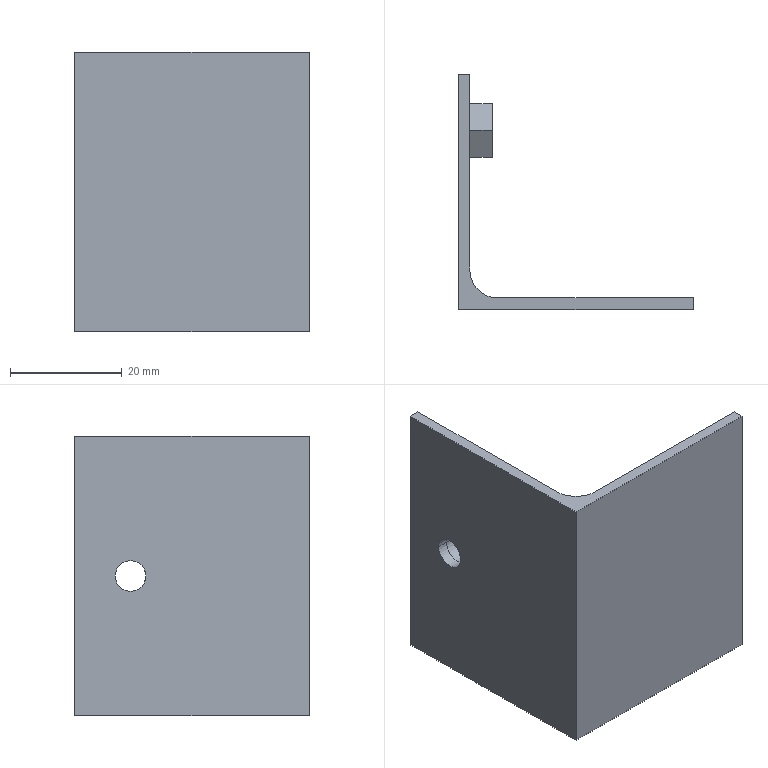Part | STEP file | ASND-0110-E63-HLTP01 control board connecting block | 2 solids | 21 faces | box 42 x 42 x 50 mm | volume 8638 mm3 | plane 16 | cylinder 5 | commonest cylinder face diameters 5.495 x2 5.5 x2 10 x1
STEP:
#1=CARTESIAN_POINT('',(0.,0.,0.));
#2=DIRECTION('',(0.,0.,1.));
#3=DIRECTION('',(1.,0.,0.));
#4=AXIS2_PLACEMENT_3D('',#1,#2,#3);
#5=CARTESIAN_POINT('',(-2.,32.75,25.));
#6=VERTEX_POINT('',#5);
#7=CARTESIAN_POINT('',(0.,32.75,25.));
#8=VERTEX_POINT('',#7);
#9=CARTESIAN_POINT('',(-10.,32.75,25.));
#10=DIRECTION('',(1.,0.,0.));
#11=VECTOR('',#10,1.);
#12=LINE('',#9,#11);
#13=CARTESIAN_POINT('',(-10.,30.,25.));
#14=DIRECTION('',(1.,0.,0.));
#15=DIRECTION('',(0.,1.,0.));
#16=AXIS2_PLACEMENT_3D('',#13,#14,#15);
#17=CYLINDRICAL_SURFACE('',#16,2.75);
#18=CARTESIAN_POINT('',(6.283,0.));
#19=DIRECTION('',(0.,1.));
#20=VECTOR('',#19,1.);
#21=LINE('',#18,#20);
#22=(GEOMETRIC_REPRESENTATION_CONTEXT(2)PARAMETRIC_REPRESENTATION_CONTEXT()REPRESENTATION_CONTEXT('',''));
#23=DEFINITIONAL_REPRESENTATION('',(#21),#22);
#24=PCURVE('',#17,#23);
#25=CARTESIAN_POINT('',(-10.,30.,25.));
#26=DIRECTION('',(1.,0.,0.));
#27=DIRECTION('',(0.,1.,0.));
#28=AXIS2_PLACEMENT_3D('',#25,#26,#27);
#29=CYLINDRICAL_SURFACE('',#28,2.75);
#30=CARTESIAN_POINT('',(0.,0.));
#31=DIRECTION('',(0.,1.));
#32=VECTOR('',#31,1.);
#33=LINE('',#30,#32);
#34=(GEOMETRIC_REPRESENTATION_CONTEXT(2)PARAMETRIC_REPRESENTATION_CONTEXT()REPRESENTATION_CONTEXT('',''));
#35=DEFINITIONAL_REPRESENTATION('',(#33),#34);
#36=PCURVE('',#29,#35);
#37=SURFACE_CURVE('',#12,(#24,#36),.PCURVE_S1.);
#38=EDGE_CURVE('',#6,#8,#37,.T.);
#39=ORIENTED_EDGE('',*,*,#38,.T.);
#40=CARTESIAN_POINT('',(0.,27.25,25.));
#41=VERTEX_POINT('',#40);
#42=CARTESIAN_POINT('',(0.,30.,25.));
#43=DIRECTION('',(1.,0.,0.));
#44=DIRECTION('',(0.,1.,0.));
#45=AXIS2_PLACEMENT_3D('',#42,#43,#44);
#46=CIRCLE('',#45,2.75);
#47=CARTESIAN_POINT('',(0.,10.));
#48=DIRECTION('',(1.,0.));
#49=VECTOR('',#48,1.);
#50=LINE('',#47,#49);
#51=(GEOMETRIC_REPRESENTATION_CONTEXT(2)PARAMETRIC_REPRESENTATION_CONTEXT()REPRESENTATION_CONTEXT('',''));
#52=DEFINITIONAL_REPRESENTATION('',(#50),#51);
#53=PCURVE('',#17,#52);
#54=CARTESIAN_POINT('',(0.,40.,50.));
#55=DIRECTION('',(1.,0.,0.));
#56=DIRECTION('',(0.,0.7071,0.7071));
#57=AXIS2_PLACEMENT_3D('',#54,#55,#56);
#58=PLANE('',#57);
#59=CARTESIAN_POINT('',(-24.749,-10.607));
#60=DIRECTION('',(0.7071,-0.7071));
#61=AXIS2_PLACEMENT_2D('',#59,#60);
#62=CIRCLE('',#61,2.75);
#63=(GEOMETRIC_REPRESENTATION_CONTEXT(2)PARAMETRIC_REPRESENTATION_CONTEXT()REPRESENTATION_CONTEXT('',''));
#64=DEFINITIONAL_REPRESENTATION('',(#62),#63);
#65=PCURVE('',#58,#64);
#66=SURFACE_CURVE('',#46,(#53,#65),.PCURVE_S1.);
#67=EDGE_CURVE('',#41,#8,#66,.T.);
#68=ORIENTED_EDGE('',*,*,#67,.F.);
#69=CARTESIAN_POINT('',(-2.,27.25,25.));
#70=VERTEX_POINT('',#69);
#71=CARTESIAN_POINT('',(-10.,27.25,25.));
#72=DIRECTION('',(1.,0.,0.));
#73=VECTOR('',#72,1.);
#74=LINE('',#71,#73);
#75=CARTESIAN_POINT('',(3.142,0.));
#76=DIRECTION('',(0.,1.));
#77=VECTOR('',#76,1.);
#78=LINE('',#75,#77);
#79=(GEOMETRIC_REPRESENTATION_CONTEXT(2)PARAMETRIC_REPRESENTATION_CONTEXT()REPRESENTATION_CONTEXT('',''));
#80=DEFINITIONAL_REPRESENTATION('',(#78),#79);
#81=PCURVE('',#17,#80);
#82=CARTESIAN_POINT('',(3.142,0.));
#83=DIRECTION('',(0.,1.));
#84=VECTOR('',#83,1.);
#85=LINE('',#82,#84);
#86=(GEOMETRIC_REPRESENTATION_CONTEXT(2)PARAMETRIC_REPRESENTATION_CONTEXT()REPRESENTATION_CONTEXT('',''));
#87=DEFINITIONAL_REPRESENTATION('',(#85),#86);
#88=PCURVE('',#29,#87);
#89=SURFACE_CURVE('',#74,(#81,#88),.PCURVE_S1.);
#90=EDGE_CURVE('',#70,#41,#89,.T.);
#91=ORIENTED_EDGE('',*,*,#90,.F.);
#92=CARTESIAN_POINT('',(-2.,30.,25.));
#93=DIRECTION('',(1.,0.,0.));
#94=DIRECTION('',(0.,1.,0.));
#95=AXIS2_PLACEMENT_3D('',#92,#93,#94);
#96=CIRCLE('',#95,2.75);
#97=CARTESIAN_POINT('',(0.,8.));
#98=DIRECTION('',(1.,0.));
#99=VECTOR('',#98,1.);
#100=LINE('',#97,#99);
#101=(GEOMETRIC_REPRESENTATION_CONTEXT(2)PARAMETRIC_REPRESENTATION_CONTEXT()REPRESENTATION_CONTEXT('',''));
#102=DEFINITIONAL_REPRESENTATION('',(#100),#101);
#103=PCURVE('',#17,#102);
#104=CARTESIAN_POINT('',(-2.,40.,50.));
#105=DIRECTION('',(1.,0.,0.));
#106=DIRECTION('',(0.,0.7071,0.7071));
#107=AXIS2_PLACEMENT_3D('',#104,#105,#106);
#108=PLANE('',#107);
#109=CARTESIAN_POINT('',(-24.749,-10.607));
#110=DIRECTION('',(0.7071,-0.7071));
#111=AXIS2_PLACEMENT_2D('',#109,#110);
#112=CIRCLE('',#111,2.75);
#113=(GEOMETRIC_REPRESENTATION_CONTEXT(2)PARAMETRIC_REPRESENTATION_CONTEXT()REPRESENTATION_CONTEXT('',''));
#114=DEFINITIONAL_REPRESENTATION('',(#112),#113);
#115=PCURVE('',#108,#114);
#116=SURFACE_CURVE('',#96,(#103,#115),.PCURVE_S1.);
#117=EDGE_CURVE('',#70,#6,#116,.T.);
#118=ORIENTED_EDGE('',*,*,#117,.T.);
#119=EDGE_LOOP('',(#39,#68,#91,#118));
#120=FACE_BOUND('',#119,.F.);
#121=ADVANCED_FACE('',(#120),#17,.F.);
#122=CARTESIAN_POINT('',(-2.,-2.,0.));
#123=VERTEX_POINT('',#122);
#124=CARTESIAN_POINT('',(40.,-2.,0.));
#125=VERTEX_POINT('',#124);
#126=CARTESIAN_POINT('',(-2.,-2.,0.));
#127=DIRECTION('',(1.,0.,0.));
#128=VECTOR('',#127,1.);
#129=LINE('',#126,#128);
#130=CARTESIAN_POINT('',(0.,-2.,50.));
#131=DIRECTION('',(0.,1.,0.));
#132=DIRECTION('',(0.7071,0.,0.7071));
#133=AXIS2_PLACEMENT_3D('',#130,#131,#132);
#134=PLANE('',#133);
#135=CARTESIAN_POINT('',(-36.77,33.941));
#136=DIRECTION('',(0.7071,0.7071));
#137=VECTOR('',#136,1.);
#138=LINE('',#135,#137);
#139=(GEOMETRIC_REPRESENTATION_CONTEXT(2)PARAMETRIC_REPRESENTATION_CONTEXT()REPRESENTATION_CONTEXT('',''));
#140=DEFINITIONAL_REPRESENTATION('',(#138),#139);
#141=PCURVE('',#134,#140);
#142=CARTESIAN_POINT('',(0.,0.,0.));
#143=DIRECTION('',(0.,0.,-1.));
#144=DIRECTION('',(0.7071,0.7071,0.));
#145=AXIS2_PLACEMENT_3D('',#142,#143,#144);
#146=PLANE('',#145);
#147=CARTESIAN_POINT('',(-2.828,0.));
#148=DIRECTION('',(0.7071,0.7071));
#149=VECTOR('',#148,1.);
#150=LINE('',#147,#149);
#151=(GEOMETRIC_REPRESENTATION_CONTEXT(2)PARAMETRIC_REPRESENTATION_CONTEXT()REPRESENTATION_CONTEXT('',''));
#152=DEFINITIONAL_REPRESENTATION('',(#150),#151);
#153=PCURVE('',#146,#152);
#154=SURFACE_CURVE('',#129,(#141,#153),.PCURVE_S1.);
#155=EDGE_CURVE('',#123,#125,#154,.T.);
#156=ORIENTED_EDGE('',*,*,#155,.T.);
#157=CARTESIAN_POINT('',(40.,-2.,50.));
#158=VERTEX_POINT('',#157);
#159=CARTESIAN_POINT('',(40.,-2.,50.));
#160=DIRECTION('',(0.,0.,-1.));
#161=VECTOR('',#160,1.);
#162=LINE('',#159,#161);
#163=CARTESIAN_POINT('',(28.284,28.284));
#164=DIRECTION('',(-0.7071,0.7071));
#165=VECTOR('',#164,1.);
#166=LINE('',#163,#165);
#167=(GEOMETRIC_REPRESENTATION_CONTEXT(2)PARAMETRIC_REPRESENTATION_CONTEXT()REPRESENTATION_CONTEXT('',''));
#168=DEFINITIONAL_REPRESENTATION('',(#166),#167);
#169=PCURVE('',#134,#168);
#170=CARTESIAN_POINT('',(40.,0.,50.));
#171=DIRECTION('',(1.,0.,0.));
#172=DIRECTION('',(0.,0.7071,0.7071));
#173=AXIS2_PLACEMENT_3D('',#170,#171,#172);
#174=PLANE('',#173);
#175=CARTESIAN_POINT('',(-1.414,1.414));
#176=DIRECTION('',(-0.7071,-0.7071));
#177=VECTOR('',#176,1.);
#178=LINE('',#175,#177);
#179=(GEOMETRIC_REPRESENTATION_CONTEXT(2)PARAMETRIC_REPRESENTATION_CONTEXT()REPRESENTATION_CONTEXT('',''));
#180=DEFINITIONAL_REPRESENTATION('',(#178),#179);
#181=PCURVE('',#174,#180);
#182=SURFACE_CURVE('',#162,(#169,#181),.PCURVE_S1.);
#183=EDGE_CURVE('',#158,#125,#182,.T.);
#184=ORIENTED_EDGE('',*,*,#183,.F.);
#185=CARTESIAN_POINT('',(-2.,-2.,50.));
#186=VERTEX_POINT('',#185);
#187=CARTESIAN_POINT('',(-2.,-2.,50.));
#188=DIRECTION('',(1.,0.,0.));
#189=VECTOR('',#188,1.);
#190=LINE('',#187,#189);
#191=CARTESIAN_POINT('',(-1.414,-1.414));
#192=DIRECTION('',(0.7071,0.7071));
#193=VECTOR('',#192,1.);
#194=LINE('',#191,#193);
#195=(GEOMETRIC_REPRESENTATION_CONTEXT(2)PARAMETRIC_REPRESENTATION_CONTEXT()REPRESENTATION_CONTEXT('',''));
#196=DEFINITIONAL_REPRESENTATION('',(#194),#195);
#197=PCURVE('',#134,#196);
#198=CARTESIAN_POINT('',(0.,0.,50.));
#199=DIRECTION('',(0.,0.,-1.));
#200=DIRECTION('',(0.7071,0.7071,0.));
#201=AXIS2_PLACEMENT_3D('',#198,#199,#200);
#202=PLANE('',#201);
#203=CARTESIAN_POINT('',(-2.828,0.));
#204=DIRECTION('',(0.7071,0.7071));
#205=VECTOR('',#204,1.);
#206=LINE('',#203,#205);
#207=(GEOMETRIC_REPRESENTATION_CONTEXT(2)PARAMETRIC_REPRESENTATION_CONTEXT()REPRESENTATION_CONTEXT('',''));
#208=DEFINITIONAL_REPRESENTATION('',(#206),#207);
#209=PCURVE('',#202,#208);
#210=SURFACE_CURVE('',#190,(#197,#209),.PCURVE_S1.);
#211=EDGE_CURVE('',#186,#158,#210,.T.);
#212=ORIENTED_EDGE('',*,*,#211,.F.);
#213=CARTESIAN_POINT('',(-2.,-2.,50.));
#214=DIRECTION('',(0.,0.,-1.));
#215=VECTOR('',#214,1.);
#216=LINE('',#213,#215);
#217=CARTESIAN_POINT('',(-1.414,-1.414));
#218=DIRECTION('',(-0.7071,0.7071));
#219=VECTOR('',#218,1.);
#220=LINE('',#217,#219);
#221=(GEOMETRIC_REPRESENTATION_CONTEXT(2)PARAMETRIC_REPRESENTATION_CONTEXT()REPRESENTATION_CONTEXT('',''));
#222=DEFINITIONAL_REPRESENTATION('',(#220),#221);
#223=PCURVE('',#134,#222);
#224=CARTESIAN_POINT('',(-29.698,29.698));
#225=DIRECTION('',(-0.7071,-0.7071));
#226=VECTOR('',#225,1.);
#227=LINE('',#224,#226);
#228=(GEOMETRIC_REPRESENTATION_CONTEXT(2)PARAMETRIC_REPRESENTATION_CONTEXT()REPRESENTATION_CONTEXT('',''));
#229=DEFINITIONAL_REPRESENTATION('',(#227),#228);
#230=PCURVE('',#108,#229);
#231=SURFACE_CURVE('',#216,(#223,#230),.PCURVE_S1.);
#232=EDGE_CURVE('',#186,#123,#231,.T.);
#233=ORIENTED_EDGE('',*,*,#232,.T.);
#234=EDGE_LOOP('',(#156,#184,#212,#233));
#235=FACE_BOUND('',#234,.T.);
#236=ADVANCED_FACE('',(#235),#134,.F.);
#237=CARTESIAN_POINT('',(40.,0.,0.));
#238=VERTEX_POINT('',#237);
#239=CARTESIAN_POINT('',(40.,0.,0.));
#240=DIRECTION('',(0.,-1.,0.));
#241=VECTOR('',#240,1.);
#242=LINE('',#239,#241);
#243=CARTESIAN_POINT('',(-35.355,-35.355));
#244=DIRECTION('',(-0.7071,0.7071));
#245=VECTOR('',#244,1.);
#246=LINE('',#243,#245);
#247=(GEOMETRIC_REPRESENTATION_CONTEXT(2)PARAMETRIC_REPRESENTATION_CONTEXT()REPRESENTATION_CONTEXT('',''));
#248=DEFINITIONAL_REPRESENTATION('',(#246),#247);
#249=PCURVE('',#174,#248);
#250=CARTESIAN_POINT('',(28.284,28.284));
#251=DIRECTION('',(-0.7071,0.7071));
#252=VECTOR('',#251,1.);
#253=LINE('',#250,#252);
#254=(GEOMETRIC_REPRESENTATION_CONTEXT(2)PARAMETRIC_REPRESENTATION_CONTEXT()REPRESENTATION_CONTEXT('',''));
#255=DEFINITIONAL_REPRESENTATION('',(#253),#254);
#256=PCURVE('',#146,#255);
#257=SURFACE_CURVE('',#242,(#249,#256),.PCURVE_S1.);
#258=EDGE_CURVE('',#238,#125,#257,.T.);
#259=ORIENTED_EDGE('',*,*,#258,.F.);
#260=CARTESIAN_POINT('',(40.,0.,50.));
#261=VERTEX_POINT('',#260);
#262=CARTESIAN_POINT('',(40.,0.,50.));
#263=DIRECTION('',(0.,0.,-1.));
#264=VECTOR('',#263,1.);
#265=LINE('',#262,#264);
#266=CARTESIAN_POINT('',(0.,0.));
#267=DIRECTION('',(-0.7071,-0.7071));
#268=VECTOR('',#267,1.);
#269=LINE('',#266,#268);
#270=(GEOMETRIC_REPRESENTATION_CONTEXT(2)PARAMETRIC_REPRESENTATION_CONTEXT()REPRESENTATION_CONTEXT('',''));
#271=DEFINITIONAL_REPRESENTATION('',(#269),#270);
#272=PCURVE('',#174,#271);
#273=CARTESIAN_POINT('',(0.,0.,50.));
#274=DIRECTION('',(0.,1.,0.));
#275=DIRECTION('',(0.7071,0.,0.7071));
#276=AXIS2_PLACEMENT_3D('',#273,#274,#275);
#277=PLANE('',#276);
#278=CARTESIAN_POINT('',(28.284,28.284));
#279=DIRECTION('',(-0.7071,0.7071));
#280=VECTOR('',#279,1.);
#281=LINE('',#278,#280);
#282=(GEOMETRIC_REPRESENTATION_CONTEXT(2)PARAMETRIC_REPRESENTATION_CONTEXT()REPRESENTATION_CONTEXT('',''));
#283=DEFINITIONAL_REPRESENTATION('',(#281),#282);
#284=PCURVE('',#277,#283);
#285=SURFACE_CURVE('',#265,(#272,#284),.PCURVE_S1.);
#286=EDGE_CURVE('',#261,#238,#285,.T.);
#287=ORIENTED_EDGE('',*,*,#286,.F.);
#288=CARTESIAN_POINT('',(40.,0.,50.));
#289=DIRECTION('',(0.,-1.,0.));
#290=VECTOR('',#289,1.);
#291=LINE('',#288,#290);
#292=CARTESIAN_POINT('',(0.,0.));
#293=DIRECTION('',(-0.7071,0.7071));
#294=VECTOR('',#293,1.);
#295=LINE('',#292,#294);
#296=(GEOMETRIC_REPRESENTATION_CONTEXT(2)PARAMETRIC_REPRESENTATION_CONTEXT()REPRESENTATION_CONTEXT('',''));
#297=DEFINITIONAL_REPRESENTATION('',(#295),#296);
#298=PCURVE('',#174,#297);
#299=CARTESIAN_POINT('',(28.284,28.284));
#300=DIRECTION('',(-0.7071,0.7071));
#301=VECTOR('',#300,1.);
#302=LINE('',#299,#301);
#303=(GEOMETRIC_REPRESENTATION_CONTEXT(2)PARAMETRIC_REPRESENTATION_CONTEXT()REPRESENTATION_CONTEXT('',''));
#304=DEFINITIONAL_REPRESENTATION('',(#302),#303);
#305=PCURVE('',#202,#304);
#306=SURFACE_CURVE('',#291,(#298,#305),.PCURVE_S1.);
#307=EDGE_CURVE('',#261,#158,#306,.T.);
#308=ORIENTED_EDGE('',*,*,#307,.T.);
#309=ORIENTED_EDGE('',*,*,#183,.T.);
#310=EDGE_LOOP('',(#259,#287,#308,#309));
#311=FACE_BOUND('',#310,.T.);
#312=ADVANCED_FACE('',(#311),#174,.T.);
#313=CARTESIAN_POINT('',(5.,0.,0.));
#314=VERTEX_POINT('',#313);
#315=CARTESIAN_POINT('',(5.,0.,0.));
#316=DIRECTION('',(1.,0.,0.));
#317=VECTOR('',#316,1.);
#318=LINE('',#315,#317);
#319=CARTESIAN_POINT('',(-31.82,38.891));
#320=DIRECTION('',(0.7071,0.7071));
#321=VECTOR('',#320,1.);
#322=LINE('',#319,#321);
#323=(GEOMETRIC_REPRESENTATION_CONTEXT(2)PARAMETRIC_REPRESENTATION_CONTEXT()REPRESENTATION_CONTEXT('',''));
#324=DEFINITIONAL_REPRESENTATION('',(#322),#323);
#325=PCURVE('',#277,#324);
#326=CARTESIAN_POINT('',(3.536,3.536));
#327=DIRECTION('',(0.7071,0.7071));
#328=VECTOR('',#327,1.);
#329=LINE('',#326,#328);
#330=(GEOMETRIC_REPRESENTATION_CONTEXT(2)PARAMETRIC_REPRESENTATION_CONTEXT()REPRESENTATION_CONTEXT('',''));
#331=DEFINITIONAL_REPRESENTATION('',(#329),#330);
#332=PCURVE('',#146,#331);
#333=SURFACE_CURVE('',#318,(#325,#332),.PCURVE_S1.);
#334=EDGE_CURVE('',#314,#238,#333,.T.);
#335=ORIENTED_EDGE('',*,*,#334,.F.);
#336=CARTESIAN_POINT('',(5.,0.,50.));
#337=VERTEX_POINT('',#336);
#338=CARTESIAN_POINT('',(5.,0.,50.));
#339=DIRECTION('',(0.,0.,1.));
#340=VECTOR('',#339,1.);
#341=LINE('',#338,#340);
#342=CARTESIAN_POINT('',(3.536,3.536));
#343=DIRECTION('',(0.7071,-0.7071));
#344=VECTOR('',#343,1.);
#345=LINE('',#342,#344);
#346=(GEOMETRIC_REPRESENTATION_CONTEXT(2)PARAMETRIC_REPRESENTATION_CONTEXT()REPRESENTATION_CONTEXT('',''));
#347=DEFINITIONAL_REPRESENTATION('',(#345),#346);
#348=PCURVE('',#277,#347);
#349=CARTESIAN_POINT('',(5.,5.,50.));
#350=DIRECTION('',(0.,0.,1.));
#351=DIRECTION('',(1.,0.,0.));
#352=AXIS2_PLACEMENT_3D('',#349,#350,#351);
#353=CYLINDRICAL_SURFACE('',#352,5.);
#354=CARTESIAN_POINT('',(4.712,0.));
#355=DIRECTION('',(0.,1.));
#356=VECTOR('',#355,1.);
#357=LINE('',#354,#356);
#358=(GEOMETRIC_REPRESENTATION_CONTEXT(2)PARAMETRIC_REPRESENTATION_CONTEXT()REPRESENTATION_CONTEXT('',''));
#359=DEFINITIONAL_REPRESENTATION('',(#357),#358);
#360=PCURVE('',#353,#359);
#361=SURFACE_CURVE('',#341,(#348,#360),.PCURVE_S1.);
#362=EDGE_CURVE('',#314,#337,#361,.T.);
#363=ORIENTED_EDGE('',*,*,#362,.T.);
#364=CARTESIAN_POINT('',(5.,0.,50.));
#365=DIRECTION('',(1.,0.,0.));
#366=VECTOR('',#365,1.);
#367=LINE('',#364,#366);
#368=CARTESIAN_POINT('',(3.536,3.536));
#369=DIRECTION('',(0.7071,0.7071));
#370=VECTOR('',#369,1.);
#371=LINE('',#368,#370);
#372=(GEOMETRIC_REPRESENTATION_CONTEXT(2)PARAMETRIC_REPRESENTATION_CONTEXT()REPRESENTATION_CONTEXT('',''));
#373=DEFINITIONAL_REPRESENTATION('',(#371),#372);
#374=PCURVE('',#277,#373);
#375=CARTESIAN_POINT('',(3.536,3.536));
#376=DIRECTION('',(0.7071,0.7071));
#377=VECTOR('',#376,1.);
#378=LINE('',#375,#377);
#379=(GEOMETRIC_REPRESENTATION_CONTEXT(2)PARAMETRIC_REPRESENTATION_CONTEXT()REPRESENTATION_CONTEXT('',''));
#380=DEFINITIONAL_REPRESENTATION('',(#378),#379);
#381=PCURVE('',#202,#380);
#382=SURFACE_CURVE('',#367,(#374,#381),.PCURVE_S1.);
#383=EDGE_CURVE('',#337,#261,#382,.T.);
#384=ORIENTED_EDGE('',*,*,#383,.T.);
#385=ORIENTED_EDGE('',*,*,#286,.T.);
#386=EDGE_LOOP('',(#335,#363,#384,#385));
#387=FACE_BOUND('',#386,.T.);
#388=ADVANCED_FACE('',(#387),#277,.T.);
#389=CARTESIAN_POINT('',(0.,40.,50.));
#390=VERTEX_POINT('',#389);
#391=CARTESIAN_POINT('',(0.,5.,50.));
#392=VERTEX_POINT('',#391);
#393=CARTESIAN_POINT('',(0.,40.,50.));
#394=DIRECTION('',(0.,-1.,0.));
#395=VECTOR('',#394,1.);
#396=LINE('',#393,#395);
#397=CARTESIAN_POINT('',(0.,0.));
#398=DIRECTION('',(-0.7071,0.7071));
#399=VECTOR('',#398,1.);
#400=LINE('',#397,#399);
#401=(GEOMETRIC_REPRESENTATION_CONTEXT(2)PARAMETRIC_REPRESENTATION_CONTEXT()REPRESENTATION_CONTEXT('',''));
#402=DEFINITIONAL_REPRESENTATION('',(#400),#401);
#403=PCURVE('',#58,#402);
#404=CARTESIAN_POINT('',(28.284,-28.284));
#405=DIRECTION('',(-0.7071,0.7071));
#406=VECTOR('',#405,1.);
#407=LINE('',#404,#406);
#408=(GEOMETRIC_REPRESENTATION_CONTEXT(2)PARAMETRIC_REPRESENTATION_CONTEXT()REPRESENTATION_CONTEXT('',''));
#409=DEFINITIONAL_REPRESENTATION('',(#407),#408);
#410=PCURVE('',#202,#409);
#411=SURFACE_CURVE('',#396,(#403,#410),.PCURVE_S1.);
#412=EDGE_CURVE('',#390,#392,#411,.T.);
#413=ORIENTED_EDGE('',*,*,#412,.T.);
#414=CARTESIAN_POINT('',(0.,5.,0.));
#415=VERTEX_POINT('',#414);
#416=CARTESIAN_POINT('',(0.,5.,50.));
#417=DIRECTION('',(0.,0.,-1.));
#418=VECTOR('',#417,1.);
#419=LINE('',#416,#418);
#420=CARTESIAN_POINT('',(-24.749,24.749));
#421=DIRECTION('',(-0.7071,-0.7071));
#422=VECTOR('',#421,1.);
#423=LINE('',#420,#422);
#424=(GEOMETRIC_REPRESENTATION_CONTEXT(2)PARAMETRIC_REPRESENTATION_CONTEXT()REPRESENTATION_CONTEXT('',''));
#425=DEFINITIONAL_REPRESENTATION('',(#423),#424);
#426=PCURVE('',#58,#425);
#427=CARTESIAN_POINT('',(3.142,0.));
#428=DIRECTION('',(0.,-1.));
#429=VECTOR('',#428,1.);
#430=LINE('',#427,#429);
#431=(GEOMETRIC_REPRESENTATION_CONTEXT(2)PARAMETRIC_REPRESENTATION_CONTEXT()REPRESENTATION_CONTEXT('',''));
#432=DEFINITIONAL_REPRESENTATION('',(#430),#431);
#433=PCURVE('',#353,#432);
#434=SURFACE_CURVE('',#419,(#426,#433),.PCURVE_S1.);
#435=EDGE_CURVE('',#392,#415,#434,.T.);
#436=ORIENTED_EDGE('',*,*,#435,.T.);
#437=CARTESIAN_POINT('',(0.,40.,0.));
#438=VERTEX_POINT('',#437);
#439=CARTESIAN_POINT('',(0.,40.,0.));
#440=DIRECTION('',(0.,-1.,0.));
#441=VECTOR('',#440,1.);
#442=LINE('',#439,#441);
#443=CARTESIAN_POINT('',(-35.355,-35.355));
#444=DIRECTION('',(-0.7071,0.7071));
#445=VECTOR('',#444,1.);
#446=LINE('',#443,#445);
#447=(GEOMETRIC_REPRESENTATION_CONTEXT(2)PARAMETRIC_REPRESENTATION_CONTEXT()REPRESENTATION_CONTEXT('',''));
#448=DEFINITIONAL_REPRESENTATION('',(#446),#447);
#449=PCURVE('',#58,#448);
#450=CARTESIAN_POINT('',(28.284,-28.284));
#451=DIRECTION('',(-0.7071,0.7071));
#452=VECTOR('',#451,1.);
#453=LINE('',#450,#452);
#454=(GEOMETRIC_REPRESENTATION_CONTEXT(2)PARAMETRIC_REPRESENTATION_CONTEXT()REPRESENTATION_CONTEXT('',''));
#455=DEFINITIONAL_REPRESENTATION('',(#453),#454);
#456=PCURVE('',#146,#455);
#457=SURFACE_CURVE('',#442,(#449,#456),.PCURVE_S1.);
#458=EDGE_CURVE('',#438,#415,#457,.T.);
#459=ORIENTED_EDGE('',*,*,#458,.F.);
#460=CARTESIAN_POINT('',(0.,40.,50.));
#461=DIRECTION('',(0.,0.,-1.));
#462=VECTOR('',#461,1.);
#463=LINE('',#460,#462);
#464=CARTESIAN_POINT('',(0.,0.));
#465=DIRECTION('',(-0.7071,-0.7071));
#466=VECTOR('',#465,1.);
#467=LINE('',#464,#466);
#468=(GEOMETRIC_REPRESENTATION_CONTEXT(2)PARAMETRIC_REPRESENTATION_CONTEXT()REPRESENTATION_CONTEXT('',''));
#469=DEFINITIONAL_REPRESENTATION('',(#467),#468);
#470=PCURVE('',#58,#469);
#471=CARTESIAN_POINT('',(-2.,40.,50.));
#472=DIRECTION('',(0.,1.,0.));
#473=DIRECTION('',(0.7071,0.,0.7071));
#474=AXIS2_PLACEMENT_3D('',#471,#472,#473);
#475=PLANE('',#474);
#476=CARTESIAN_POINT('',(1.414,1.414));
#477=DIRECTION('',(-0.7071,0.7071));
#478=VECTOR('',#477,1.);
#479=LINE('',#476,#478);
#480=(GEOMETRIC_REPRESENTATION_CONTEXT(2)PARAMETRIC_REPRESENTATION_CONTEXT()REPRESENTATION_CONTEXT('',''));
#481=DEFINITIONAL_REPRESENTATION('',(#479),#480);
#482=PCURVE('',#475,#481);
#483=SURFACE_CURVE('',#463,(#470,#482),.PCURVE_S1.);
#484=EDGE_CURVE('',#390,#438,#483,.T.);
#485=ORIENTED_EDGE('',*,*,#484,.F.);
#486=EDGE_LOOP('',(#413,#436,#459,#485));
#487=FACE_BOUND('',#486,.T.);
#488=CARTESIAN_POINT('',(0.,30.,25.));
#489=DIRECTION('',(1.,0.,0.));
#490=DIRECTION('',(0.,1.,0.));
#491=AXIS2_PLACEMENT_3D('',#488,#489,#490);
#492=CIRCLE('',#491,2.75);
#493=CARTESIAN_POINT('',(-24.749,-10.607));
#494=DIRECTION('',(0.7071,-0.7071));
#495=AXIS2_PLACEMENT_2D('',#493,#494);
#496=CIRCLE('',#495,2.75);
#497=(GEOMETRIC_REPRESENTATION_CONTEXT(2)PARAMETRIC_REPRESENTATION_CONTEXT()REPRESENTATION_CONTEXT('',''));
#498=DEFINITIONAL_REPRESENTATION('',(#496),#497);
#499=PCURVE('',#58,#498);
#500=CARTESIAN_POINT('',(0.,10.));
#501=DIRECTION('',(1.,0.));
#502=VECTOR('',#501,1.);
#503=LINE('',#500,#502);
#504=(GEOMETRIC_REPRESENTATION_CONTEXT(2)PARAMETRIC_REPRESENTATION_CONTEXT()REPRESENTATION_CONTEXT('',''));
#505=DEFINITIONAL_REPRESENTATION('',(#503),#504);
#506=PCURVE('',#29,#505);
#507=SURFACE_CURVE('',#492,(#499,#506),.PCURVE_S1.);
#508=EDGE_CURVE('',#8,#41,#507,.T.);
#509=ORIENTED_EDGE('',*,*,#508,.F.);
#510=ORIENTED_EDGE('',*,*,#67,.F.);
#511=EDGE_LOOP('',(#509,#510));
#512=FACE_BOUND('',#511,.T.);
#513=ADVANCED_FACE('',(#487,#512),#58,.T.);
#514=CARTESIAN_POINT('',(-2.,40.,0.));
#515=VERTEX_POINT('',#514);
#516=CARTESIAN_POINT('',(-2.,40.,0.));
#517=DIRECTION('',(1.,0.,0.));
#518=VECTOR('',#517,1.);
#519=LINE('',#516,#518);
#520=CARTESIAN_POINT('',(-35.355,35.355));
#521=DIRECTION('',(0.7071,0.7071));
#522=VECTOR('',#521,1.);
#523=LINE('',#520,#522);
#524=(GEOMETRIC_REPRESENTATION_CONTEXT(2)PARAMETRIC_REPRESENTATION_CONTEXT()REPRESENTATION_CONTEXT('',''));
#525=DEFINITIONAL_REPRESENTATION('',(#523),#524);
#526=PCURVE('',#475,#525);
#527=CARTESIAN_POINT('',(26.87,-29.698));
#528=DIRECTION('',(0.7071,0.7071));
#529=VECTOR('',#528,1.);
#530=LINE('',#527,#529);
#531=(GEOMETRIC_REPRESENTATION_CONTEXT(2)PARAMETRIC_REPRESENTATION_CONTEXT()REPRESENTATION_CONTEXT('',''));
#532=DEFINITIONAL_REPRESENTATION('',(#530),#531);
#533=PCURVE('',#146,#532);
#534=SURFACE_CURVE('',#519,(#526,#533),.PCURVE_S1.);
#535=EDGE_CURVE('',#515,#438,#534,.T.);
#536=ORIENTED_EDGE('',*,*,#535,.F.);
#537=CARTESIAN_POINT('',(-2.,40.,50.));
#538=VERTEX_POINT('',#537);
#539=CARTESIAN_POINT('',(-2.,40.,50.));
#540=DIRECTION('',(0.,0.,-1.));
#541=VECTOR('',#540,1.);
#542=LINE('',#539,#541);
#543=CARTESIAN_POINT('',(0.,0.));
#544=DIRECTION('',(-0.7071,0.7071));
#545=VECTOR('',#544,1.);
#546=LINE('',#543,#545);
#547=(GEOMETRIC_REPRESENTATION_CONTEXT(2)PARAMETRIC_REPRESENTATION_CONTEXT()REPRESENTATION_CONTEXT('',''));
#548=DEFINITIONAL_REPRESENTATION('',(#546),#547);
#549=PCURVE('',#475,#548);
#550=CARTESIAN_POINT('',(0.,0.));
#551=DIRECTION('',(-0.7071,-0.7071));
#552=VECTOR('',#551,1.);
#553=LINE('',#550,#552);
#554=(GEOMETRIC_REPRESENTATION_CONTEXT(2)PARAMETRIC_REPRESENTATION_CONTEXT()REPRESENTATION_CONTEXT('',''));
#555=DEFINITIONAL_REPRESENTATION('',(#553),#554);
#556=PCURVE('',#108,#555);
#557=SURFACE_CURVE('',#542,(#549,#556),.PCURVE_S1.);
#558=EDGE_CURVE('',#538,#515,#557,.T.);
#559=ORIENTED_EDGE('',*,*,#558,.F.);
#560=CARTESIAN_POINT('',(-2.,40.,50.));
#561=DIRECTION('',(1.,0.,0.));
#562=VECTOR('',#561,1.);
#563=LINE('',#560,#562);
#564=CARTESIAN_POINT('',(0.,0.));
#565=DIRECTION('',(0.7071,0.7071));
#566=VECTOR('',#565,1.);
#567=LINE('',#564,#566);
#568=(GEOMETRIC_REPRESENTATION_CONTEXT(2)PARAMETRIC_REPRESENTATION_CONTEXT()REPRESENTATION_CONTEXT('',''));
#569=DEFINITIONAL_REPRESENTATION('',(#567),#568);
#570=PCURVE('',#475,#569);
#571=CARTESIAN_POINT('',(26.87,-29.698));
#572=DIRECTION('',(0.7071,0.7071));
#573=VECTOR('',#572,1.);
#574=LINE('',#571,#573);
#575=(GEOMETRIC_REPRESENTATION_CONTEXT(2)PARAMETRIC_REPRESENTATION_CONTEXT()REPRESENTATION_CONTEXT('',''));
#576=DEFINITIONAL_REPRESENTATION('',(#574),#575);
#577=PCURVE('',#202,#576);
#578=SURFACE_CURVE('',#563,(#570,#577),.PCURVE_S1.);
#579=EDGE_CURVE('',#538,#390,#578,.T.);
#580=ORIENTED_EDGE('',*,*,#579,.T.);
#581=ORIENTED_EDGE('',*,*,#484,.T.);
#582=EDGE_LOOP('',(#536,#559,#580,#581));
#583=FACE_BOUND('',#582,.T.);
#584=ADVANCED_FACE('',(#583),#475,.T.);
#585=CARTESIAN_POINT('',(-2.,40.,0.));
#586=DIRECTION('',(0.,-1.,0.));
#587=VECTOR('',#586,1.);
#588=LINE('',#585,#587);
#589=CARTESIAN_POINT('',(-35.355,-35.355));
#590=DIRECTION('',(-0.7071,0.7071));
#591=VECTOR('',#590,1.);
#592=LINE('',#589,#591);
#593=(GEOMETRIC_REPRESENTATION_CONTEXT(2)PARAMETRIC_REPRESENTATION_CONTEXT()REPRESENTATION_CONTEXT('',''));
#594=DEFINITIONAL_REPRESENTATION('',(#592),#593);
#595=PCURVE('',#108,#594);
#596=CARTESIAN_POINT('',(26.87,-29.698));
#597=DIRECTION('',(-0.7071,0.7071));
#598=VECTOR('',#597,1.);
#599=LINE('',#596,#598);
#600=(GEOMETRIC_REPRESENTATION_CONTEXT(2)PARAMETRIC_REPRESENTATION_CONTEXT()REPRESENTATION_CONTEXT('',''));
#601=DEFINITIONAL_REPRESENTATION('',(#599),#600);
#602=PCURVE('',#146,#601);
#603=SURFACE_CURVE('',#588,(#595,#602),.PCURVE_S1.);
#604=EDGE_CURVE('',#515,#123,#603,.T.);
#605=ORIENTED_EDGE('',*,*,#604,.T.);
#606=ORIENTED_EDGE('',*,*,#232,.F.);
#607=CARTESIAN_POINT('',(-2.,40.,50.));
#608=DIRECTION('',(0.,-1.,0.));
#609=VECTOR('',#608,1.);
#610=LINE('',#607,#609);
#611=CARTESIAN_POINT('',(0.,0.));
#612=DIRECTION('',(-0.7071,0.7071));
#613=VECTOR('',#612,1.);
#614=LINE('',#611,#613);
#615=(GEOMETRIC_REPRESENTATION_CONTEXT(2)PARAMETRIC_REPRESENTATION_CONTEXT()REPRESENTATION_CONTEXT('',''));
#616=DEFINITIONAL_REPRESENTATION('',(#614),#615);
#617=PCURVE('',#108,#616);
#618=CARTESIAN_POINT('',(26.87,-29.698));
#619=DIRECTION('',(-0.7071,0.7071));
#620=VECTOR('',#619,1.);
#621=LINE('',#618,#620);
#622=(GEOMETRIC_REPRESENTATION_CONTEXT(2)PARAMETRIC_REPRESENTATION_CONTEXT()REPRESENTATION_CONTEXT('',''));
#623=DEFINITIONAL_REPRESENTATION('',(#621),#622);
#624=PCURVE('',#202,#623);
#625=SURFACE_CURVE('',#610,(#617,#624),.PCURVE_S1.);
#626=EDGE_CURVE('',#538,#186,#625,.T.);
#627=ORIENTED_EDGE('',*,*,#626,.F.);
#628=ORIENTED_EDGE('',*,*,#558,.T.);
#629=EDGE_LOOP('',(#605,#606,#627,#628));
#630=FACE_BOUND('',#629,.T.);
#631=CARTESIAN_POINT('',(-2.,30.,25.));
#632=DIRECTION('',(1.,0.,0.));
#633=DIRECTION('',(0.,1.,0.));
#634=AXIS2_PLACEMENT_3D('',#631,#632,#633);
#635=CIRCLE('',#634,2.75);
#636=CARTESIAN_POINT('',(-24.749,-10.607));
#637=DIRECTION('',(0.7071,-0.7071));
#638=AXIS2_PLACEMENT_2D('',#636,#637);
#639=CIRCLE('',#638,2.75);
#640=(GEOMETRIC_REPRESENTATION_CONTEXT(2)PARAMETRIC_REPRESENTATION_CONTEXT()REPRESENTATION_CONTEXT('',''));
#641=DEFINITIONAL_REPRESENTATION('',(#639),#640);
#642=PCURVE('',#108,#641);
#643=CARTESIAN_POINT('',(0.,8.));
#644=DIRECTION('',(1.,0.));
#645=VECTOR('',#644,1.);
#646=LINE('',#643,#645);
#647=(GEOMETRIC_REPRESENTATION_CONTEXT(2)PARAMETRIC_REPRESENTATION_CONTEXT()REPRESENTATION_CONTEXT('',''));
#648=DEFINITIONAL_REPRESENTATION('',(#646),#647);
#649=PCURVE('',#29,#648);
#650=SURFACE_CURVE('',#635,(#642,#649),.PCURVE_S1.);
#651=EDGE_CURVE('',#6,#70,#650,.T.);
#652=ORIENTED_EDGE('',*,*,#651,.T.);
#653=ORIENTED_EDGE('',*,*,#117,.T.);
#654=EDGE_LOOP('',(#652,#653));
#655=FACE_BOUND('',#654,.T.);
#656=ADVANCED_FACE('',(#630,#655),#108,.F.);
#657=ORIENTED_EDGE('',*,*,#211,.T.);
#658=ORIENTED_EDGE('',*,*,#307,.F.);
#659=ORIENTED_EDGE('',*,*,#383,.F.);
#660=CARTESIAN_POINT('',(5.,5.,50.));
#661=DIRECTION('',(0.,0.,-1.));
#662=DIRECTION('',(-1.,0.,0.));
#663=AXIS2_PLACEMENT_3D('',#660,#661,#662);
#664=CIRCLE('',#663,5.);
#665=CARTESIAN_POINT('',(7.071,0.));
#666=DIRECTION('',(-0.7071,-0.7071));
#667=AXIS2_PLACEMENT_2D('',#665,#666);
#668=CIRCLE('',#667,5.);
#669=(GEOMETRIC_REPRESENTATION_CONTEXT(2)PARAMETRIC_REPRESENTATION_CONTEXT()REPRESENTATION_CONTEXT('',''));
#670=DEFINITIONAL_REPRESENTATION('',(#668),#669);
#671=PCURVE('',#202,#670);
#672=CARTESIAN_POINT('',(9.425,0.));
#673=DIRECTION('',(-1.,0.));
#674=VECTOR('',#673,1.);
#675=LINE('',#672,#674);
#676=(GEOMETRIC_REPRESENTATION_CONTEXT(2)PARAMETRIC_REPRESENTATION_CONTEXT()REPRESENTATION_CONTEXT('',''));
#677=DEFINITIONAL_REPRESENTATION('',(#675),#676);
#678=PCURVE('',#353,#677);
#679=SURFACE_CURVE('',#664,(#671,#678),.PCURVE_S1.);
#680=EDGE_CURVE('',#337,#392,#679,.T.);
#681=ORIENTED_EDGE('',*,*,#680,.T.);
#682=ORIENTED_EDGE('',*,*,#412,.F.);
#683=ORIENTED_EDGE('',*,*,#579,.F.);
#684=ORIENTED_EDGE('',*,*,#626,.T.);
#685=EDGE_LOOP('',(#657,#658,#659,#681,#682,#683,#684));
#686=FACE_BOUND('',#685,.T.);
#687=ADVANCED_FACE('',(#686),#202,.F.);
#688=ORIENTED_EDGE('',*,*,#155,.F.);
#689=ORIENTED_EDGE('',*,*,#604,.F.);
#690=ORIENTED_EDGE('',*,*,#535,.T.);
#691=ORIENTED_EDGE('',*,*,#458,.T.);
#692=CARTESIAN_POINT('',(5.,5.,0.));
#693=DIRECTION('',(0.,0.,1.));
#694=DIRECTION('',(-1.,0.,0.));
#695=AXIS2_PLACEMENT_3D('',#692,#693,#694);
#696=CIRCLE('',#695,5.);
#697=CARTESIAN_POINT('',(3.536,-3.536));
#698=CARTESIAN_POINT('',(-2.588,2.588));
#699=CARTESIAN_POINT('',(5.777,4.83));
#700=CARTESIAN_POINT('',(14.142,7.071));
#701=CARTESIAN_POINT('',(11.901,-1.294));
#702=CARTESIAN_POINT('',(9.659,-9.659));
#703=CARTESIAN_POINT('',(3.536,-3.536));
#704=(BOUNDED_CURVE()B_SPLINE_CURVE(2,(#697,#698,#699,#700,#701,#702,#703),.UNSPECIFIED.,.T.,.F.)B_SPLINE_CURVE_WITH_KNOTS((1,2,2,2,2,1),(-2.094,0.,2.094,4.189,6.283,8.378),.UNSPECIFIED.)CURVE()GEOMETRIC_REPRESENTATION_ITEM()RATIONAL_B_SPLINE_CURVE((1.,0.5,1.,0.5,1.,0.5,1.))REPRESENTATION_ITEM(''));
#705=(GEOMETRIC_REPRESENTATION_CONTEXT(2)PARAMETRIC_REPRESENTATION_CONTEXT()REPRESENTATION_CONTEXT('',''));
#706=DEFINITIONAL_REPRESENTATION('',(#704),#705);
#707=PCURVE('',#146,#706);
#708=CARTESIAN_POINT('',(3.142,-50.));
#709=DIRECTION('',(1.,0.));
#710=VECTOR('',#709,1.);
#711=LINE('',#708,#710);
#712=(GEOMETRIC_REPRESENTATION_CONTEXT(2)PARAMETRIC_REPRESENTATION_CONTEXT()REPRESENTATION_CONTEXT('',''));
#713=DEFINITIONAL_REPRESENTATION('',(#711),#712);
#714=PCURVE('',#353,#713);
#715=SURFACE_CURVE('',#696,(#707,#714),.PCURVE_S1.);
#716=EDGE_CURVE('',#415,#314,#715,.T.);
#717=ORIENTED_EDGE('',*,*,#716,.T.);
#718=ORIENTED_EDGE('',*,*,#334,.T.);
#719=ORIENTED_EDGE('',*,*,#258,.T.);
#720=EDGE_LOOP('',(#688,#689,#690,#691,#717,#718,#719));
#721=FACE_BOUND('',#720,.T.);
#722=ADVANCED_FACE('',(#721),#146,.T.);
#723=ORIENTED_EDGE('',*,*,#435,.T.);
#724=ORIENTED_EDGE('',*,*,#716,.T.);
#725=ORIENTED_EDGE('',*,*,#362,.T.);
#726=ORIENTED_EDGE('',*,*,#680,.T.);
#727=EDGE_LOOP('',(#723,#724,#725,#726));
#728=FACE_BOUND('',#727,.F.);
#729=ADVANCED_FACE('',(#728),#353,.F.);
#730=ORIENTED_EDGE('',*,*,#508,.F.);
#731=ORIENTED_EDGE('',*,*,#38,.F.);
#732=ORIENTED_EDGE('',*,*,#651,.T.);
#733=ORIENTED_EDGE('',*,*,#90,.T.);
#734=EDGE_LOOP('',(#730,#731,#732,#733));
#735=FACE_BOUND('',#734,.F.);
#736=ADVANCED_FACE('',(#735),#29,.F.);
#737=CLOSED_SHELL('',(#121,#236,#312,#388,#513,#584,#656,#687,#722,#729,#736));
#738=MANIFOLD_SOLID_BREP('',#737);
#739=CARTESIAN_POINT('',(4.,27.253,25.));
#740=VERTEX_POINT('',#739);
#741=CARTESIAN_POINT('',(0.,27.253,25.));
#742=VERTEX_POINT('',#741);
#743=CARTESIAN_POINT('',(4.,27.253,25.));
#744=DIRECTION('',(-1.,0.,0.));
#745=VECTOR('',#744,1.);
#746=LINE('',#743,#745);
#747=CARTESIAN_POINT('',(4.,30.,25.));
#748=DIRECTION('',(-1.,0.,0.));
#749=DIRECTION('',(0.,-1.,0.));
#750=AXIS2_PLACEMENT_3D('',#747,#748,#749);
#751=CYLINDRICAL_SURFACE('',#750,2.748);
#752=CARTESIAN_POINT('',(6.283,0.));
#753=DIRECTION('',(0.,1.));
#754=VECTOR('',#753,1.);
#755=LINE('',#752,#754);
#756=(GEOMETRIC_REPRESENTATION_CONTEXT(2)PARAMETRIC_REPRESENTATION_CONTEXT()REPRESENTATION_CONTEXT('',''));
#757=DEFINITIONAL_REPRESENTATION('',(#755),#756);
#758=PCURVE('',#751,#757);
#759=CARTESIAN_POINT('',(4.,30.,25.));
#760=DIRECTION('',(-1.,0.,0.));
#761=DIRECTION('',(0.,-1.,0.));
#762=AXIS2_PLACEMENT_3D('',#759,#760,#761);
#763=CYLINDRICAL_SURFACE('',#762,2.748);
#764=CARTESIAN_POINT('',(0.,0.));
#765=DIRECTION('',(0.,1.));
#766=VECTOR('',#765,1.);
#767=LINE('',#764,#766);
#768=(GEOMETRIC_REPRESENTATION_CONTEXT(2)PARAMETRIC_REPRESENTATION_CONTEXT()REPRESENTATION_CONTEXT('',''));
#769=DEFINITIONAL_REPRESENTATION('',(#767),#768);
#770=PCURVE('',#763,#769);
#771=SURFACE_CURVE('',#746,(#758,#770),.PCURVE_S1.);
#772=EDGE_CURVE('',#740,#742,#771,.T.);
#773=ORIENTED_EDGE('',*,*,#772,.T.);
#774=CARTESIAN_POINT('',(0.,32.748,25.));
#775=VERTEX_POINT('',#774);
#776=CARTESIAN_POINT('',(0.,30.,25.));
#777=DIRECTION('',(1.,0.,0.));
#778=DIRECTION('',(0.,1.,0.));
#779=AXIS2_PLACEMENT_3D('',#776,#777,#778);
#780=CIRCLE('',#779,2.748);
#781=CARTESIAN_POINT('',(9.425,4.));
#782=DIRECTION('',(-1.,0.));
#783=VECTOR('',#782,1.);
#784=LINE('',#781,#783);
#785=(GEOMETRIC_REPRESENTATION_CONTEXT(2)PARAMETRIC_REPRESENTATION_CONTEXT()REPRESENTATION_CONTEXT('',''));
#786=DEFINITIONAL_REPRESENTATION('',(#784),#785);
#787=PCURVE('',#751,#786);
#788=CARTESIAN_POINT('',(0.,0.,0.));
#789=DIRECTION('',(1.,0.,0.));
#790=DIRECTION('',(0.,0.7071,0.7071));
#791=AXIS2_PLACEMENT_3D('',#788,#789,#790);
#792=PLANE('',#791);
#793=CARTESIAN_POINT('',(38.891,-3.536));
#794=DIRECTION('',(0.7071,-0.7071));
#795=AXIS2_PLACEMENT_2D('',#793,#794);
#796=CIRCLE('',#795,2.748);
#797=(GEOMETRIC_REPRESENTATION_CONTEXT(2)PARAMETRIC_REPRESENTATION_CONTEXT()REPRESENTATION_CONTEXT('',''));
#798=DEFINITIONAL_REPRESENTATION('',(#796),#797);
#799=PCURVE('',#792,#798);
#800=SURFACE_CURVE('',#780,(#787,#799),.PCURVE_S1.);
#801=EDGE_CURVE('',#742,#775,#800,.T.);
#802=ORIENTED_EDGE('',*,*,#801,.T.);
#803=CARTESIAN_POINT('',(4.,32.748,25.));
#804=VERTEX_POINT('',#803);
#805=CARTESIAN_POINT('',(4.,32.748,25.));
#806=DIRECTION('',(-1.,0.,0.));
#807=VECTOR('',#806,1.);
#808=LINE('',#805,#807);
#809=CARTESIAN_POINT('',(3.142,0.));
#810=DIRECTION('',(0.,1.));
#811=VECTOR('',#810,1.);
#812=LINE('',#809,#811);
#813=(GEOMETRIC_REPRESENTATION_CONTEXT(2)PARAMETRIC_REPRESENTATION_CONTEXT()REPRESENTATION_CONTEXT('',''));
#814=DEFINITIONAL_REPRESENTATION('',(#812),#813);
#815=PCURVE('',#751,#814);
#816=CARTESIAN_POINT('',(3.142,0.));
#817=DIRECTION('',(0.,1.));
#818=VECTOR('',#817,1.);
#819=LINE('',#816,#818);
#820=(GEOMETRIC_REPRESENTATION_CONTEXT(2)PARAMETRIC_REPRESENTATION_CONTEXT()REPRESENTATION_CONTEXT('',''));
#821=DEFINITIONAL_REPRESENTATION('',(#819),#820);
#822=PCURVE('',#763,#821);
#823=SURFACE_CURVE('',#808,(#815,#822),.PCURVE_S1.);
#824=EDGE_CURVE('',#804,#775,#823,.T.);
#825=ORIENTED_EDGE('',*,*,#824,.F.);
#826=CARTESIAN_POINT('',(4.,30.,25.));
#827=DIRECTION('',(1.,0.,0.));
#828=DIRECTION('',(0.,1.,0.));
#829=AXIS2_PLACEMENT_3D('',#826,#827,#828);
#830=CIRCLE('',#829,2.748);
#831=CARTESIAN_POINT('',(9.425,0.));
#832=DIRECTION('',(-1.,0.));
#833=VECTOR('',#832,1.);
#834=LINE('',#831,#833);
#835=(GEOMETRIC_REPRESENTATION_CONTEXT(2)PARAMETRIC_REPRESENTATION_CONTEXT()REPRESENTATION_CONTEXT('',''));
#836=DEFINITIONAL_REPRESENTATION('',(#834),#835);
#837=PCURVE('',#751,#836);
#838=CARTESIAN_POINT('',(4.,0.,0.));
#839=DIRECTION('',(1.,0.,0.));
#840=DIRECTION('',(0.,0.7071,0.7071));
#841=AXIS2_PLACEMENT_3D('',#838,#839,#840);
#842=PLANE('',#841);
#843=CARTESIAN_POINT('',(38.891,-3.536));
#844=DIRECTION('',(0.7071,-0.7071));
#845=AXIS2_PLACEMENT_2D('',#843,#844);
#846=CIRCLE('',#845,2.748);
#847=(GEOMETRIC_REPRESENTATION_CONTEXT(2)PARAMETRIC_REPRESENTATION_CONTEXT()REPRESENTATION_CONTEXT('',''));
#848=DEFINITIONAL_REPRESENTATION('',(#846),#847);
#849=PCURVE('',#842,#848);
#850=SURFACE_CURVE('',#830,(#837,#849),.PCURVE_S1.);
#851=EDGE_CURVE('',#740,#804,#850,.T.);
#852=ORIENTED_EDGE('',*,*,#851,.F.);
#853=EDGE_LOOP('',(#773,#802,#825,#852));
#854=FACE_BOUND('',#853,.F.);
#855=ADVANCED_FACE('',(#854),#751,.F.);
#856=CARTESIAN_POINT('',(4.,30.,19.518));
#857=VERTEX_POINT('',#856);
#858=CARTESIAN_POINT('',(4.,34.748,22.259));
#859=VERTEX_POINT('',#858);
#860=CARTESIAN_POINT('',(4.,30.,19.518));
#861=DIRECTION('',(0.,0.866,0.5));
#862=VECTOR('',#861,1.);
#863=LINE('',#860,#862);
#864=CARTESIAN_POINT('',(35.015,-7.412));
#865=DIRECTION('',(0.9659,-0.2588));
#866=VECTOR('',#865,1.);
#867=LINE('',#864,#866);
#868=(GEOMETRIC_REPRESENTATION_CONTEXT(2)PARAMETRIC_REPRESENTATION_CONTEXT()REPRESENTATION_CONTEXT('',''));
#869=DEFINITIONAL_REPRESENTATION('',(#867),#868);
#870=PCURVE('',#842,#869);
#871=CARTESIAN_POINT('',(4.,30.,19.518));
#872=DIRECTION('',(0.,-0.5,0.866));
#873=DIRECTION('',(0.4472,0.7746,0.4472));
#874=AXIS2_PLACEMENT_3D('',#871,#872,#873);
#875=PLANE('',#874);
#876=CARTESIAN_POINT('',(0.,0.));
#877=DIRECTION('',(0.8944,0.4472));
#878=VECTOR('',#877,1.);
#879=LINE('',#876,#878);
#880=(GEOMETRIC_REPRESENTATION_CONTEXT(2)PARAMETRIC_REPRESENTATION_CONTEXT()REPRESENTATION_CONTEXT('',''));
#881=DEFINITIONAL_REPRESENTATION('',(#879),#880);
#882=PCURVE('',#875,#881);
#883=SURFACE_CURVE('',#863,(#870,#882),.PCURVE_S1.);
#884=EDGE_CURVE('',#857,#859,#883,.T.);
#885=ORIENTED_EDGE('',*,*,#884,.T.);
#886=CARTESIAN_POINT('',(4.,34.748,27.741));
#887=VERTEX_POINT('',#886);
#888=CARTESIAN_POINT('',(4.,34.748,22.259));
#889=DIRECTION('',(0.,0.,1.));
#890=VECTOR('',#889,1.);
#891=LINE('',#888,#890);
#892=CARTESIAN_POINT('',(40.31,-8.831));
#893=DIRECTION('',(0.7071,0.7071));
#894=VECTOR('',#893,1.);
#895=LINE('',#892,#894);
#896=(GEOMETRIC_REPRESENTATION_CONTEXT(2)PARAMETRIC_REPRESENTATION_CONTEXT()REPRESENTATION_CONTEXT('',''));
#897=DEFINITIONAL_REPRESENTATION('',(#895),#896);
#898=PCURVE('',#842,#897);
#899=CARTESIAN_POINT('',(4.,34.748,22.259));
#900=DIRECTION('',(0.,-1.,0.));
#901=DIRECTION('',(0.7071,0.,0.7071));
#902=AXIS2_PLACEMENT_3D('',#899,#900,#901);
#903=PLANE('',#902);
#904=CARTESIAN_POINT('',(0.,0.));
#905=DIRECTION('',(0.7071,0.7071));
#906=VECTOR('',#905,1.);
#907=LINE('',#904,#906);
#908=(GEOMETRIC_REPRESENTATION_CONTEXT(2)PARAMETRIC_REPRESENTATION_CONTEXT()REPRESENTATION_CONTEXT('',''));
#909=DEFINITIONAL_REPRESENTATION('',(#907),#908);
#910=PCURVE('',#903,#909);
#911=SURFACE_CURVE('',#891,(#898,#910),.PCURVE_S1.);
#912=EDGE_CURVE('',#859,#887,#911,.T.);
#913=ORIENTED_EDGE('',*,*,#912,.T.);
#914=CARTESIAN_POINT('',(4.,30.,30.482));
#915=VERTEX_POINT('',#914);
#916=CARTESIAN_POINT('',(4.,34.748,27.741));
#917=DIRECTION('',(0.,-0.866,0.5));
#918=VECTOR('',#917,1.);
#919=LINE('',#916,#918);
#920=CARTESIAN_POINT('',(44.186,-4.954));
#921=DIRECTION('',(-0.2588,0.9659));
#922=VECTOR('',#921,1.);
#923=LINE('',#920,#922);
#924=(GEOMETRIC_REPRESENTATION_CONTEXT(2)PARAMETRIC_REPRESENTATION_CONTEXT()REPRESENTATION_CONTEXT('',''));
#925=DEFINITIONAL_REPRESENTATION('',(#923),#924);
#926=PCURVE('',#842,#925);
#927=CARTESIAN_POINT('',(4.,34.748,27.741));
#928=DIRECTION('',(0.,-0.5,-0.866));
#929=DIRECTION('',(0.6547,0.6547,-0.378));
#930=AXIS2_PLACEMENT_3D('',#927,#928,#929);
#931=PLANE('',#930);
#932=CARTESIAN_POINT('',(0.,0.));
#933=DIRECTION('',(-0.7559,0.6547));
#934=VECTOR('',#933,1.);
#935=LINE('',#932,#934);
#936=(GEOMETRIC_REPRESENTATION_CONTEXT(2)PARAMETRIC_REPRESENTATION_CONTEXT()REPRESENTATION_CONTEXT('',''));
#937=DEFINITIONAL_REPRESENTATION('',(#935),#936);
#938=PCURVE('',#931,#937);
#939=SURFACE_CURVE('',#919,(#926,#938),.PCURVE_S1.);
#940=EDGE_CURVE('',#887,#915,#939,.T.);
#941=ORIENTED_EDGE('',*,*,#940,.T.);
#942=CARTESIAN_POINT('',(4.,25.253,27.741));
#943=VERTEX_POINT('',#942);
#944=CARTESIAN_POINT('',(4.,30.,30.482));
#945=DIRECTION('',(0.,-0.866,-0.5));
#946=VECTOR('',#945,1.);
#947=LINE('',#944,#946);
#948=CARTESIAN_POINT('',(42.767,0.3408));
#949=DIRECTION('',(-0.9659,0.2588));
#950=VECTOR('',#949,1.);
#951=LINE('',#948,#950);
#952=(GEOMETRIC_REPRESENTATION_CONTEXT(2)PARAMETRIC_REPRESENTATION_CONTEXT()REPRESENTATION_CONTEXT('',''));
#953=DEFINITIONAL_REPRESENTATION('',(#951),#952);
#954=PCURVE('',#842,#953);
#955=CARTESIAN_POINT('',(4.,30.,30.482));
#956=DIRECTION('',(0.,0.5,-0.866));
#957=DIRECTION('',(0.6547,0.6547,0.378));
#958=AXIS2_PLACEMENT_3D('',#955,#956,#957);
#959=PLANE('',#958);
#960=CARTESIAN_POINT('',(0.,0.));
#961=DIRECTION('',(-0.7559,0.6547));
#962=VECTOR('',#961,1.);
#963=LINE('',#960,#962);
#964=(GEOMETRIC_REPRESENTATION_CONTEXT(2)PARAMETRIC_REPRESENTATION_CONTEXT()REPRESENTATION_CONTEXT('',''));
#965=DEFINITIONAL_REPRESENTATION('',(#963),#964);
#966=PCURVE('',#959,#965);
#967=SURFACE_CURVE('',#947,(#954,#966),.PCURVE_S1.);
#968=EDGE_CURVE('',#915,#943,#967,.T.);
#969=ORIENTED_EDGE('',*,*,#968,.T.);
#970=CARTESIAN_POINT('',(4.,25.253,22.259));
#971=VERTEX_POINT('',#970);
#972=CARTESIAN_POINT('',(4.,25.253,27.741));
#973=DIRECTION('',(0.,0.,-1.));
#974=VECTOR('',#973,1.);
#975=LINE('',#972,#974);
#976=CARTESIAN_POINT('',(37.472,1.76));
#977=DIRECTION('',(-0.7071,-0.7071));
#978=VECTOR('',#977,1.);
#979=LINE('',#976,#978);
#980=(GEOMETRIC_REPRESENTATION_CONTEXT(2)PARAMETRIC_REPRESENTATION_CONTEXT()REPRESENTATION_CONTEXT('',''));
#981=DEFINITIONAL_REPRESENTATION('',(#979),#980);
#982=PCURVE('',#842,#981);
#983=CARTESIAN_POINT('',(4.,25.253,27.741));
#984=DIRECTION('',(0.,1.,0.));
#985=DIRECTION('',(0.7071,0.,0.7071));
#986=AXIS2_PLACEMENT_3D('',#983,#984,#985);
#987=PLANE('',#986);
#988=CARTESIAN_POINT('',(0.,0.));
#989=DIRECTION('',(-0.7071,0.7071));
#990=VECTOR('',#989,1.);
#991=LINE('',#988,#990);
#992=(GEOMETRIC_REPRESENTATION_CONTEXT(2)PARAMETRIC_REPRESENTATION_CONTEXT()REPRESENTATION_CONTEXT('',''));
#993=DEFINITIONAL_REPRESENTATION('',(#991),#992);
#994=PCURVE('',#987,#993);
#995=SURFACE_CURVE('',#975,(#982,#994),.PCURVE_S1.);
#996=EDGE_CURVE('',#943,#971,#995,.T.);
#997=ORIENTED_EDGE('',*,*,#996,.T.);
#998=CARTESIAN_POINT('',(4.,25.253,22.259));
#999=DIRECTION('',(0.,0.866,-0.5));
#1000=VECTOR('',#999,1.);
#1001=LINE('',#998,#1000);
#1002=CARTESIAN_POINT('',(33.596,-2.117));
#1003=DIRECTION('',(0.2588,-0.9659));
#1004=VECTOR('',#1003,1.);
#1005=LINE('',#1002,#1004);
#1006=(GEOMETRIC_REPRESENTATION_CONTEXT(2)PARAMETRIC_REPRESENTATION_CONTEXT()REPRESENTATION_CONTEXT('',''));
#1007=DEFINITIONAL_REPRESENTATION('',(#1005),#1006);
#1008=PCURVE('',#842,#1007);
#1009=CARTESIAN_POINT('',(4.,25.253,22.259));
#1010=DIRECTION('',(0.,0.5,0.866));
#1011=DIRECTION('',(0.6547,0.6547,-0.378));
#1012=AXIS2_PLACEMENT_3D('',#1009,#1010,#1011);
#1013=PLANE('',#1012);
#1014=CARTESIAN_POINT('',(0.,0.));
#1015=DIRECTION('',(0.7559,0.6547));
#1016=VECTOR('',#1015,1.);
#1017=LINE('',#1014,#1016);
#1018=(GEOMETRIC_REPRESENTATION_CONTEXT(2)PARAMETRIC_REPRESENTATION_CONTEXT()REPRESENTATION_CONTEXT('',''));
#1019=DEFINITIONAL_REPRESENTATION('',(#1017),#1018);
#1020=PCURVE('',#1013,#1019);
#1021=SURFACE_CURVE('',#1001,(#1008,#1020),.PCURVE_S1.);
#1022=EDGE_CURVE('',#971,#857,#1021,.T.);
#1023=ORIENTED_EDGE('',*,*,#1022,.T.);
#1024=EDGE_LOOP('',(#885,#913,#941,#969,#997,#1023));
#1025=FACE_BOUND('',#1024,.T.);
#1026=ORIENTED_EDGE('',*,*,#851,.F.);
#1027=CARTESIAN_POINT('',(4.,30.,25.));
#1028=DIRECTION('',(1.,0.,0.));
#1029=DIRECTION('',(0.,1.,0.));
#1030=AXIS2_PLACEMENT_3D('',#1027,#1028,#1029);
#1031=CIRCLE('',#1030,2.748);
#1032=CARTESIAN_POINT('',(38.891,-3.536));
#1033=DIRECTION('',(0.7071,-0.7071));
#1034=AXIS2_PLACEMENT_2D('',#1032,#1033);
#1035=CIRCLE('',#1034,2.748);
#1036=(GEOMETRIC_REPRESENTATION_CONTEXT(2)PARAMETRIC_REPRESENTATION_CONTEXT()REPRESENTATION_CONTEXT('',''));
#1037=DEFINITIONAL_REPRESENTATION('',(#1035),#1036);
#1038=PCURVE('',#842,#1037);
#1039=CARTESIAN_POINT('',(3.142,0.));
#1040=DIRECTION('',(-1.,0.));
#1041=VECTOR('',#1040,1.);
#1042=LINE('',#1039,#1041);
#1043=(GEOMETRIC_REPRESENTATION_CONTEXT(2)PARAMETRIC_REPRESENTATION_CONTEXT()REPRESENTATION_CONTEXT('',''));
#1044=DEFINITIONAL_REPRESENTATION('',(#1042),#1043);
#1045=PCURVE('',#763,#1044);
#1046=SURFACE_CURVE('',#1031,(#1038,#1045),.PCURVE_S1.);
#1047=EDGE_CURVE('',#804,#740,#1046,.T.);
#1048=ORIENTED_EDGE('',*,*,#1047,.F.);
#1049=EDGE_LOOP('',(#1026,#1048));
#1050=FACE_BOUND('',#1049,.T.);
#1051=ADVANCED_FACE('',(#1025,#1050),#842,.T.);
#1052=CARTESIAN_POINT('',(0.,30.,19.518));
#1053=VERTEX_POINT('',#1052);
#1054=CARTESIAN_POINT('',(0.,34.748,22.259));
#1055=VERTEX_POINT('',#1054);
#1056=CARTESIAN_POINT('',(0.,30.,19.518));
#1057=DIRECTION('',(0.,0.866,0.5));
#1058=VECTOR('',#1057,1.);
#1059=LINE('',#1056,#1058);
#1060=CARTESIAN_POINT('',(35.015,-7.412));
#1061=DIRECTION('',(0.9659,-0.2588));
#1062=VECTOR('',#1061,1.);
#1063=LINE('',#1060,#1062);
#1064=(GEOMETRIC_REPRESENTATION_CONTEXT(2)PARAMETRIC_REPRESENTATION_CONTEXT()REPRESENTATION_CONTEXT('',''));
#1065=DEFINITIONAL_REPRESENTATION('',(#1063),#1064);
#1066=PCURVE('',#792,#1065);
#1067=CARTESIAN_POINT('',(-1.789,3.578));
#1068=DIRECTION('',(0.8944,0.4472));
#1069=VECTOR('',#1068,1.);
#1070=LINE('',#1067,#1069);
#1071=(GEOMETRIC_REPRESENTATION_CONTEXT(2)PARAMETRIC_REPRESENTATION_CONTEXT()REPRESENTATION_CONTEXT('',''));
#1072=DEFINITIONAL_REPRESENTATION('',(#1070),#1071);
#1073=PCURVE('',#875,#1072);
#1074=SURFACE_CURVE('',#1059,(#1066,#1073),.PCURVE_S1.);
#1075=EDGE_CURVE('',#1053,#1055,#1074,.T.);
#1076=ORIENTED_EDGE('',*,*,#1075,.F.);
#1077=CARTESIAN_POINT('',(0.,25.253,22.259));
#1078=VERTEX_POINT('',#1077);
#1079=CARTESIAN_POINT('',(0.,25.253,22.259));
#1080=DIRECTION('',(0.,0.866,-0.5));
#1081=VECTOR('',#1080,1.);
#1082=LINE('',#1079,#1081);
#1083=CARTESIAN_POINT('',(33.596,-2.117));
#1084=DIRECTION('',(0.2588,-0.9659));
#1085=VECTOR('',#1084,1.);
#1086=LINE('',#1083,#1085);
#1087=(GEOMETRIC_REPRESENTATION_CONTEXT(2)PARAMETRIC_REPRESENTATION_CONTEXT()REPRESENTATION_CONTEXT('',''));
#1088=DEFINITIONAL_REPRESENTATION('',(#1086),#1087);
#1089=PCURVE('',#792,#1088);
#1090=CARTESIAN_POINT('',(-2.619,3.024));
#1091=DIRECTION('',(0.7559,0.6547));
#1092=VECTOR('',#1091,1.);
#1093=LINE('',#1090,#1092);
#1094=(GEOMETRIC_REPRESENTATION_CONTEXT(2)PARAMETRIC_REPRESENTATION_CONTEXT()REPRESENTATION_CONTEXT('',''));
#1095=DEFINITIONAL_REPRESENTATION('',(#1093),#1094);
#1096=PCURVE('',#1013,#1095);
#1097=SURFACE_CURVE('',#1082,(#1089,#1096),.PCURVE_S1.);
#1098=EDGE_CURVE('',#1078,#1053,#1097,.T.);
#1099=ORIENTED_EDGE('',*,*,#1098,.F.);
#1100=CARTESIAN_POINT('',(0.,25.253,27.741));
#1101=VERTEX_POINT('',#1100);
#1102=CARTESIAN_POINT('',(0.,25.253,27.741));
#1103=DIRECTION('',(0.,0.,-1.));
#1104=VECTOR('',#1103,1.);
#1105=LINE('',#1102,#1104);
#1106=CARTESIAN_POINT('',(37.472,1.76));
#1107=DIRECTION('',(-0.7071,-0.7071));
#1108=VECTOR('',#1107,1.);
#1109=LINE('',#1106,#1108);
#1110=(GEOMETRIC_REPRESENTATION_CONTEXT(2)PARAMETRIC_REPRESENTATION_CONTEXT()REPRESENTATION_CONTEXT('',''));
#1111=DEFINITIONAL_REPRESENTATION('',(#1109),#1110);
#1112=PCURVE('',#792,#1111);
#1113=CARTESIAN_POINT('',(-2.828,-2.828));
#1114=DIRECTION('',(-0.7071,0.7071));
#1115=VECTOR('',#1114,1.);
#1116=LINE('',#1113,#1115);
#1117=(GEOMETRIC_REPRESENTATION_CONTEXT(2)PARAMETRIC_REPRESENTATION_CONTEXT()REPRESENTATION_CONTEXT('',''));
#1118=DEFINITIONAL_REPRESENTATION('',(#1116),#1117);
#1119=PCURVE('',#987,#1118);
#1120=SURFACE_CURVE('',#1105,(#1112,#1119),.PCURVE_S1.);
#1121=EDGE_CURVE('',#1101,#1078,#1120,.T.);
#1122=ORIENTED_EDGE('',*,*,#1121,.F.);
#1123=CARTESIAN_POINT('',(0.,30.,30.482));
#1124=VERTEX_POINT('',#1123);
#1125=CARTESIAN_POINT('',(0.,30.,30.482));
#1126=DIRECTION('',(0.,-0.866,-0.5));
#1127=VECTOR('',#1126,1.);
#1128=LINE('',#1125,#1127);
#1129=CARTESIAN_POINT('',(42.767,0.3408));
#1130=DIRECTION('',(-0.9659,0.2588));
#1131=VECTOR('',#1130,1.);
#1132=LINE('',#1129,#1131);
#1133=(GEOMETRIC_REPRESENTATION_CONTEXT(2)PARAMETRIC_REPRESENTATION_CONTEXT()REPRESENTATION_CONTEXT('',''));
#1134=DEFINITIONAL_REPRESENTATION('',(#1132),#1133);
#1135=PCURVE('',#792,#1134);
#1136=CARTESIAN_POINT('',(-2.619,-3.024));
#1137=DIRECTION('',(-0.7559,0.6547));
#1138=VECTOR('',#1137,1.);
#1139=LINE('',#1136,#1138);
#1140=(GEOMETRIC_REPRESENTATION_CONTEXT(2)PARAMETRIC_REPRESENTATION_CONTEXT()REPRESENTATION_CONTEXT('',''));
#1141=DEFINITIONAL_REPRESENTATION('',(#1139),#1140);
#1142=PCURVE('',#959,#1141);
#1143=SURFACE_CURVE('',#1128,(#1135,#1142),.PCURVE_S1.);
#1144=EDGE_CURVE('',#1124,#1101,#1143,.T.);
#1145=ORIENTED_EDGE('',*,*,#1144,.F.);
#1146=CARTESIAN_POINT('',(0.,34.748,27.741));
#1147=VERTEX_POINT('',#1146);
#1148=CARTESIAN_POINT('',(0.,34.748,27.741));
#1149=DIRECTION('',(0.,-0.866,0.5));
#1150=VECTOR('',#1149,1.);
#1151=LINE('',#1148,#1150);
#1152=CARTESIAN_POINT('',(44.186,-4.954));
#1153=DIRECTION('',(-0.2588,0.9659));
#1154=VECTOR('',#1153,1.);
#1155=LINE('',#1152,#1154);
#1156=(GEOMETRIC_REPRESENTATION_CONTEXT(2)PARAMETRIC_REPRESENTATION_CONTEXT()REPRESENTATION_CONTEXT('',''));
#1157=DEFINITIONAL_REPRESENTATION('',(#1155),#1156);
#1158=PCURVE('',#792,#1157);
#1159=CARTESIAN_POINT('',(-2.619,-3.024));
#1160=DIRECTION('',(-0.7559,0.6547));
#1161=VECTOR('',#1160,1.);
#1162=LINE('',#1159,#1161);
#1163=(GEOMETRIC_REPRESENTATION_CONTEXT(2)PARAMETRIC_REPRESENTATION_CONTEXT()REPRESENTATION_CONTEXT('',''));
#1164=DEFINITIONAL_REPRESENTATION('',(#1162),#1163);
#1165=PCURVE('',#931,#1164);
#1166=SURFACE_CURVE('',#1151,(#1158,#1165),.PCURVE_S1.);
#1167=EDGE_CURVE('',#1147,#1124,#1166,.T.);
#1168=ORIENTED_EDGE('',*,*,#1167,.F.);
#1169=CARTESIAN_POINT('',(0.,34.748,22.259));
#1170=DIRECTION('',(0.,0.,1.));
#1171=VECTOR('',#1170,1.);
#1172=LINE('',#1169,#1171);
#1173=CARTESIAN_POINT('',(40.31,-8.831));
#1174=DIRECTION('',(0.7071,0.7071));
#1175=VECTOR('',#1174,1.);
#1176=LINE('',#1173,#1175);
#1177=(GEOMETRIC_REPRESENTATION_CONTEXT(2)PARAMETRIC_REPRESENTATION_CONTEXT()REPRESENTATION_CONTEXT('',''));
#1178=DEFINITIONAL_REPRESENTATION('',(#1176),#1177);
#1179=PCURVE('',#792,#1178);
#1180=CARTESIAN_POINT('',(-2.828,2.828));
#1181=DIRECTION('',(0.7071,0.7071));
#1182=VECTOR('',#1181,1.);
#1183=LINE('',#1180,#1182);
#1184=(GEOMETRIC_REPRESENTATION_CONTEXT(2)PARAMETRIC_REPRESENTATION_CONTEXT()REPRESENTATION_CONTEXT('',''));
#1185=DEFINITIONAL_REPRESENTATION('',(#1183),#1184);
#1186=PCURVE('',#903,#1185);
#1187=SURFACE_CURVE('',#1172,(#1179,#1186),.PCURVE_S1.);
#1188=EDGE_CURVE('',#1055,#1147,#1187,.T.);
#1189=ORIENTED_EDGE('',*,*,#1188,.F.);
#1190=EDGE_LOOP('',(#1076,#1099,#1122,#1145,#1168,#1189));
#1191=FACE_BOUND('',#1190,.T.);
#1192=ORIENTED_EDGE('',*,*,#801,.T.);
#1193=CARTESIAN_POINT('',(0.,30.,25.));
#1194=DIRECTION('',(1.,0.,0.));
#1195=DIRECTION('',(0.,1.,0.));
#1196=AXIS2_PLACEMENT_3D('',#1193,#1194,#1195);
#1197=CIRCLE('',#1196,2.748);
#1198=CARTESIAN_POINT('',(38.891,-3.536));
#1199=DIRECTION('',(0.7071,-0.7071));
#1200=AXIS2_PLACEMENT_2D('',#1198,#1199);
#1201=CIRCLE('',#1200,2.748);
#1202=(GEOMETRIC_REPRESENTATION_CONTEXT(2)PARAMETRIC_REPRESENTATION_CONTEXT()REPRESENTATION_CONTEXT('',''));
#1203=DEFINITIONAL_REPRESENTATION('',(#1201),#1202);
#1204=PCURVE('',#792,#1203);
#1205=CARTESIAN_POINT('',(3.142,4.));
#1206=DIRECTION('',(-1.,0.));
#1207=VECTOR('',#1206,1.);
#1208=LINE('',#1205,#1207);
#1209=(GEOMETRIC_REPRESENTATION_CONTEXT(2)PARAMETRIC_REPRESENTATION_CONTEXT()REPRESENTATION_CONTEXT('',''));
#1210=DEFINITIONAL_REPRESENTATION('',(#1208),#1209);
#1211=PCURVE('',#763,#1210);
#1212=SURFACE_CURVE('',#1197,(#1204,#1211),.PCURVE_S1.);
#1213=EDGE_CURVE('',#775,#742,#1212,.T.);
#1214=ORIENTED_EDGE('',*,*,#1213,.T.);
#1215=EDGE_LOOP('',(#1192,#1214));
#1216=FACE_BOUND('',#1215,.T.);
#1217=ADVANCED_FACE('',(#1191,#1216),#792,.F.);
#1218=ORIENTED_EDGE('',*,*,#1075,.T.);
#1219=CARTESIAN_POINT('',(4.,34.748,22.259));
#1220=DIRECTION('',(-1.,0.,0.));
#1221=VECTOR('',#1220,1.);
#1222=LINE('',#1219,#1221);
#1223=CARTESIAN_POINT('',(4.903,2.452));
#1224=DIRECTION('',(-0.4472,0.8944));
#1225=VECTOR('',#1224,1.);
#1226=LINE('',#1223,#1225);
#1227=(GEOMETRIC_REPRESENTATION_CONTEXT(2)PARAMETRIC_REPRESENTATION_CONTEXT()REPRESENTATION_CONTEXT('',''));
#1228=DEFINITIONAL_REPRESENTATION('',(#1226),#1227);
#1229=PCURVE('',#875,#1228);
#1230=CARTESIAN_POINT('',(0.,0.));
#1231=DIRECTION('',(-0.7071,0.7071));
#1232=VECTOR('',#1231,1.);
#1233=LINE('',#1230,#1232);
#1234=(GEOMETRIC_REPRESENTATION_CONTEXT(2)PARAMETRIC_REPRESENTATION_CONTEXT()REPRESENTATION_CONTEXT('',''));
#1235=DEFINITIONAL_REPRESENTATION('',(#1233),#1234);
#1236=PCURVE('',#903,#1235);
#1237=SURFACE_CURVE('',#1222,(#1229,#1236),.PCURVE_S1.);
#1238=EDGE_CURVE('',#859,#1055,#1237,.T.);
#1239=ORIENTED_EDGE('',*,*,#1238,.F.);
#1240=ORIENTED_EDGE('',*,*,#884,.F.);
#1241=CARTESIAN_POINT('',(4.,30.,19.518));
#1242=DIRECTION('',(-1.,0.,0.));
#1243=VECTOR('',#1242,1.);
#1244=LINE('',#1241,#1243);
#1245=CARTESIAN_POINT('',(0.,0.));
#1246=DIRECTION('',(-0.4472,0.8944));
#1247=VECTOR('',#1246,1.);
#1248=LINE('',#1245,#1247);
#1249=(GEOMETRIC_REPRESENTATION_CONTEXT(2)PARAMETRIC_REPRESENTATION_CONTEXT()REPRESENTATION_CONTEXT('',''));
#1250=DEFINITIONAL_REPRESENTATION('',(#1248),#1249);
#1251=PCURVE('',#875,#1250);
#1252=CARTESIAN_POINT('',(4.144,3.589));
#1253=DIRECTION('',(-0.6547,0.7559));
#1254=VECTOR('',#1253,1.);
#1255=LINE('',#1252,#1254);
#1256=(GEOMETRIC_REPRESENTATION_CONTEXT(2)PARAMETRIC_REPRESENTATION_CONTEXT()REPRESENTATION_CONTEXT('',''));
#1257=DEFINITIONAL_REPRESENTATION('',(#1255),#1256);
#1258=PCURVE('',#1013,#1257);
#1259=SURFACE_CURVE('',#1244,(#1251,#1258),.PCURVE_S1.);
#1260=EDGE_CURVE('',#857,#1053,#1259,.T.);
#1261=ORIENTED_EDGE('',*,*,#1260,.T.);
#1262=EDGE_LOOP('',(#1218,#1239,#1240,#1261));
#1263=FACE_BOUND('',#1262,.T.);
#1264=ADVANCED_FACE('',(#1263),#875,.F.);
#1265=ORIENTED_EDGE('',*,*,#1188,.T.);
#1266=CARTESIAN_POINT('',(4.,34.748,27.741));
#1267=DIRECTION('',(-1.,0.,0.));
#1268=VECTOR('',#1267,1.);
#1269=LINE('',#1266,#1268);
#1270=CARTESIAN_POINT('',(3.876,3.876));
#1271=DIRECTION('',(-0.7071,0.7071));
#1272=VECTOR('',#1271,1.);
#1273=LINE('',#1270,#1272);
#1274=(GEOMETRIC_REPRESENTATION_CONTEXT(2)PARAMETRIC_REPRESENTATION_CONTEXT()REPRESENTATION_CONTEXT('',''));
#1275=DEFINITIONAL_REPRESENTATION('',(#1273),#1274);
#1276=PCURVE('',#903,#1275);
#1277=CARTESIAN_POINT('',(0.,0.));
#1278=DIRECTION('',(-0.6547,-0.7559));
#1279=VECTOR('',#1278,1.);
#1280=LINE('',#1277,#1279);
#1281=(GEOMETRIC_REPRESENTATION_CONTEXT(2)PARAMETRIC_REPRESENTATION_CONTEXT()REPRESENTATION_CONTEXT('',''));
#1282=DEFINITIONAL_REPRESENTATION('',(#1280),#1281);
#1283=PCURVE('',#931,#1282);
#1284=SURFACE_CURVE('',#1269,(#1276,#1283),.PCURVE_S1.);
#1285=EDGE_CURVE('',#887,#1147,#1284,.T.);
#1286=ORIENTED_EDGE('',*,*,#1285,.F.);
#1287=ORIENTED_EDGE('',*,*,#912,.F.);
#1288=ORIENTED_EDGE('',*,*,#1238,.T.);
#1289=EDGE_LOOP('',(#1265,#1286,#1287,#1288));
#1290=FACE_BOUND('',#1289,.T.);
#1291=ADVANCED_FACE('',(#1290),#903,.F.);
#1292=ORIENTED_EDGE('',*,*,#1167,.T.);
#1293=CARTESIAN_POINT('',(4.,30.,30.482));
#1294=DIRECTION('',(-1.,0.,0.));
#1295=VECTOR('',#1294,1.);
#1296=LINE('',#1293,#1295);
#1297=CARTESIAN_POINT('',(-4.144,3.589));
#1298=DIRECTION('',(-0.6547,-0.7559));
#1299=VECTOR('',#1298,1.);
#1300=LINE('',#1297,#1299);
#1301=(GEOMETRIC_REPRESENTATION_CONTEXT(2)PARAMETRIC_REPRESENTATION_CONTEXT()REPRESENTATION_CONTEXT('',''));
#1302=DEFINITIONAL_REPRESENTATION('',(#1300),#1301);
#1303=PCURVE('',#931,#1302);
#1304=CARTESIAN_POINT('',(0.,0.));
#1305=DIRECTION('',(-0.6547,-0.7559));
#1306=VECTOR('',#1305,1.);
#1307=LINE('',#1304,#1306);
#1308=(GEOMETRIC_REPRESENTATION_CONTEXT(2)PARAMETRIC_REPRESENTATION_CONTEXT()REPRESENTATION_CONTEXT('',''));
#1309=DEFINITIONAL_REPRESENTATION('',(#1307),#1308);
#1310=PCURVE('',#959,#1309);
#1311=SURFACE_CURVE('',#1296,(#1303,#1310),.PCURVE_S1.);
#1312=EDGE_CURVE('',#915,#1124,#1311,.T.);
#1313=ORIENTED_EDGE('',*,*,#1312,.F.);
#1314=ORIENTED_EDGE('',*,*,#940,.F.);
#1315=ORIENTED_EDGE('',*,*,#1285,.T.);
#1316=EDGE_LOOP('',(#1292,#1313,#1314,#1315));
#1317=FACE_BOUND('',#1316,.T.);
#1318=ADVANCED_FACE('',(#1317),#931,.F.);
#1319=ORIENTED_EDGE('',*,*,#1144,.T.);
#1320=CARTESIAN_POINT('',(4.,25.253,27.741));
#1321=DIRECTION('',(-1.,0.,0.));
#1322=VECTOR('',#1321,1.);
#1323=LINE('',#1320,#1322);
#1324=CARTESIAN_POINT('',(-4.144,3.589));
#1325=DIRECTION('',(-0.6547,-0.7559));
#1326=VECTOR('',#1325,1.);
#1327=LINE('',#1324,#1326);
#1328=(GEOMETRIC_REPRESENTATION_CONTEXT(2)PARAMETRIC_REPRESENTATION_CONTEXT()REPRESENTATION_CONTEXT('',''));
#1329=DEFINITIONAL_REPRESENTATION('',(#1327),#1328);
#1330=PCURVE('',#959,#1329);
#1331=CARTESIAN_POINT('',(0.,0.));
#1332=DIRECTION('',(-0.7071,-0.7071));
#1333=VECTOR('',#1332,1.);
#1334=LINE('',#1331,#1333);
#1335=(GEOMETRIC_REPRESENTATION_CONTEXT(2)PARAMETRIC_REPRESENTATION_CONTEXT()REPRESENTATION_CONTEXT('',''));
#1336=DEFINITIONAL_REPRESENTATION('',(#1334),#1335);
#1337=PCURVE('',#987,#1336);
#1338=SURFACE_CURVE('',#1323,(#1330,#1337),.PCURVE_S1.);
#1339=EDGE_CURVE('',#943,#1101,#1338,.T.);
#1340=ORIENTED_EDGE('',*,*,#1339,.F.);
#1341=ORIENTED_EDGE('',*,*,#968,.F.);
#1342=ORIENTED_EDGE('',*,*,#1312,.T.);
#1343=EDGE_LOOP('',(#1319,#1340,#1341,#1342));
#1344=FACE_BOUND('',#1343,.T.);
#1345=ADVANCED_FACE('',(#1344),#959,.F.);
#1346=ORIENTED_EDGE('',*,*,#1121,.T.);
#1347=CARTESIAN_POINT('',(4.,25.253,22.259));
#1348=DIRECTION('',(-1.,0.,0.));
#1349=VECTOR('',#1348,1.);
#1350=LINE('',#1347,#1349);
#1351=CARTESIAN_POINT('',(-3.876,3.876));
#1352=DIRECTION('',(-0.7071,-0.7071));
#1353=VECTOR('',#1352,1.);
#1354=LINE('',#1351,#1353);
#1355=(GEOMETRIC_REPRESENTATION_CONTEXT(2)PARAMETRIC_REPRESENTATION_CONTEXT()REPRESENTATION_CONTEXT('',''));
#1356=DEFINITIONAL_REPRESENTATION('',(#1354),#1355);
#1357=PCURVE('',#987,#1356);
#1358=CARTESIAN_POINT('',(0.,0.));
#1359=DIRECTION('',(-0.6547,0.7559));
#1360=VECTOR('',#1359,1.);
#1361=LINE('',#1358,#1360);
#1362=(GEOMETRIC_REPRESENTATION_CONTEXT(2)PARAMETRIC_REPRESENTATION_CONTEXT()REPRESENTATION_CONTEXT('',''));
#1363=DEFINITIONAL_REPRESENTATION('',(#1361),#1362);
#1364=PCURVE('',#1013,#1363);
#1365=SURFACE_CURVE('',#1350,(#1357,#1364),.PCURVE_S1.);
#1366=EDGE_CURVE('',#971,#1078,#1365,.T.);
#1367=ORIENTED_EDGE('',*,*,#1366,.F.);
#1368=ORIENTED_EDGE('',*,*,#996,.F.);
#1369=ORIENTED_EDGE('',*,*,#1339,.T.);
#1370=EDGE_LOOP('',(#1346,#1367,#1368,#1369));
#1371=FACE_BOUND('',#1370,.T.);
#1372=ADVANCED_FACE('',(#1371),#987,.F.);
#1373=ORIENTED_EDGE('',*,*,#1098,.T.);
#1374=ORIENTED_EDGE('',*,*,#1260,.F.);
#1375=ORIENTED_EDGE('',*,*,#1022,.F.);
#1376=ORIENTED_EDGE('',*,*,#1366,.T.);
#1377=EDGE_LOOP('',(#1373,#1374,#1375,#1376));
#1378=FACE_BOUND('',#1377,.T.);
#1379=ADVANCED_FACE('',(#1378),#1013,.F.);
#1380=ORIENTED_EDGE('',*,*,#1213,.T.);
#1381=ORIENTED_EDGE('',*,*,#772,.F.);
#1382=ORIENTED_EDGE('',*,*,#1047,.F.);
#1383=ORIENTED_EDGE('',*,*,#824,.T.);
#1384=EDGE_LOOP('',(#1380,#1381,#1382,#1383));
#1385=FACE_BOUND('',#1384,.F.);
#1386=ADVANCED_FACE('',(#1385),#763,.F.);
#1387=CLOSED_SHELL('',(#855,#1051,#1217,#1264,#1291,#1318,#1345,#1372,#1379,#1386));
#1388=MANIFOLD_SOLID_BREP('',#1387);
#1389=(LENGTH_UNIT()NAMED_UNIT(*)SI_UNIT(.MILLI.,.METRE.));
#1390=UNCERTAINTY_MEASURE_WITH_UNIT(LENGTH_MEASURE(0.0000001),#1389,'','');
#1391=(NAMED_UNIT(*)PLANE_ANGLE_UNIT()SI_UNIT($,.RADIAN.));
#1392=(NAMED_UNIT(*)SI_UNIT($,.STERADIAN.)SOLID_ANGLE_UNIT());
#1393=(GEOMETRIC_REPRESENTATION_CONTEXT(3)GLOBAL_UNCERTAINTY_ASSIGNED_CONTEXT((#1390))GLOBAL_UNIT_ASSIGNED_CONTEXT((#1389,#1391,#1392))REPRESENTATION_CONTEXT('',''));
#1394=SHAPE_REPRESENTATION('',(#4,#738,#1388),#1393);